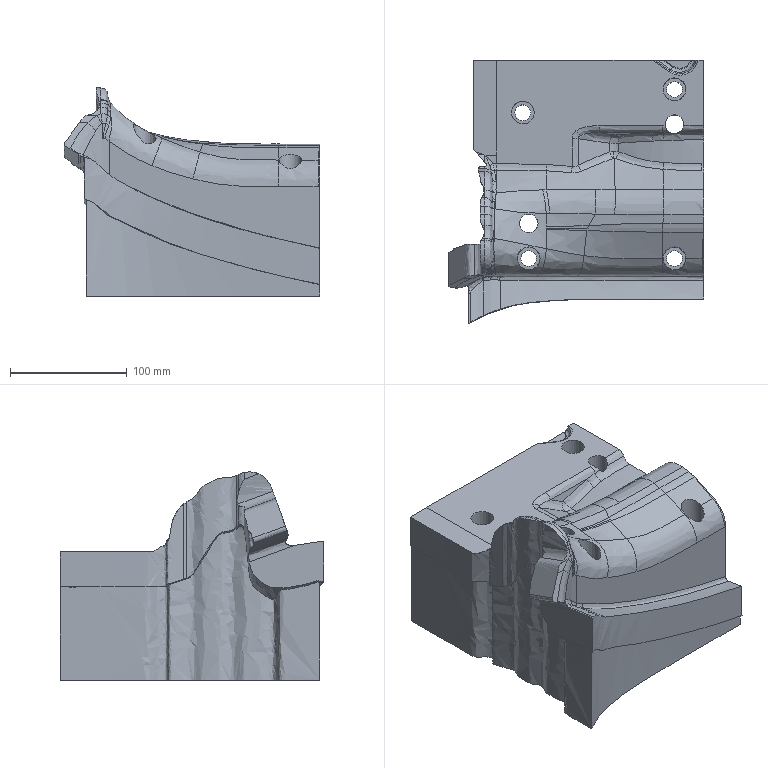Part | NX | features solid 2 | 1 solid | 186 faces | box 218.885 x 226.119 x 178.566 mm | volume 4431174 mm3 | spline 164 | plane 12 | cylinder 10 | commonest cylinder face diameters 13.5 x4 19.5 x4 16 x2